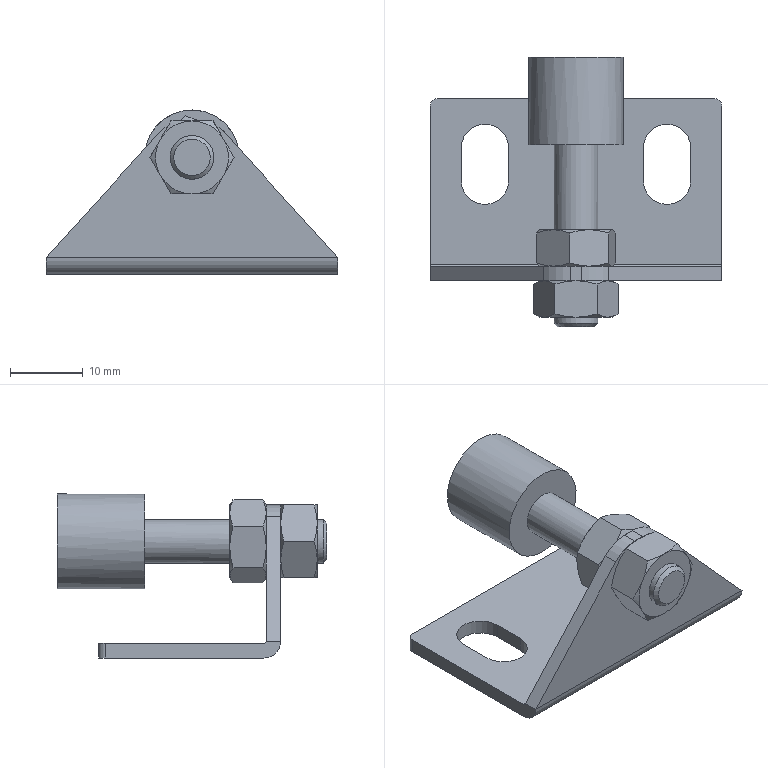Part | STEP file | 1 solid | 79 faces | box 40 x 37 x 22.5 mm | volume 5385 mm3 | plane 35 | cone 25 | cylinder 17 | torus 2 | commonest cylinder face diameters 6.5 x5 6 x3 10 x3 2 x2 0.6 x1 4.6 x1